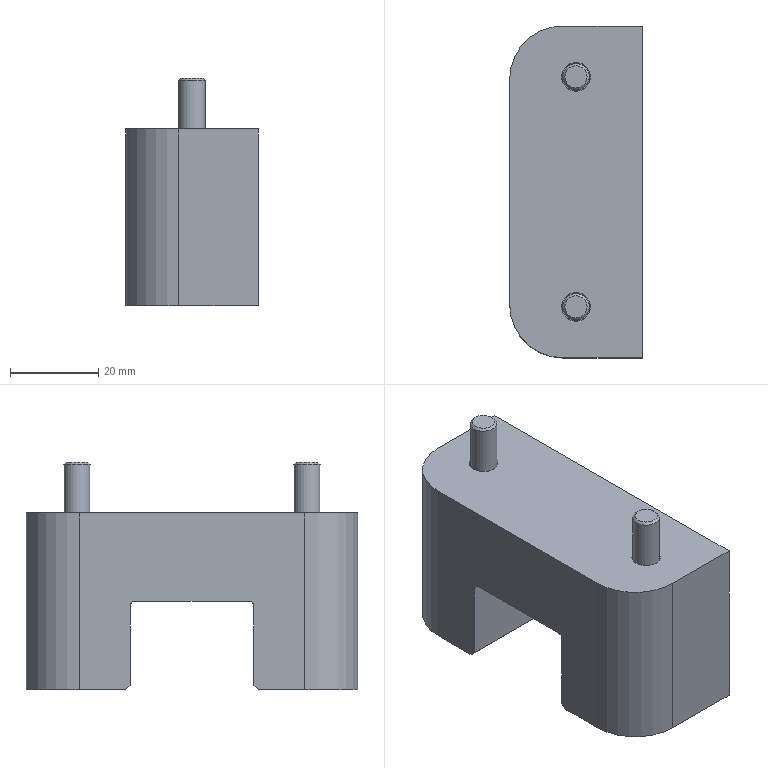Part | STEP file | LKM-Top Locks-TOP_75-A | 3 solids | 52 faces | box 30 x 75 x 51.5 mm | volume 70556 mm3 | plane 34 | cylinder 14 | cone 4 | commonest cylinder face diameters 6.5 x3 11 x3 2 x2 6 x2 10 x2 24 x2